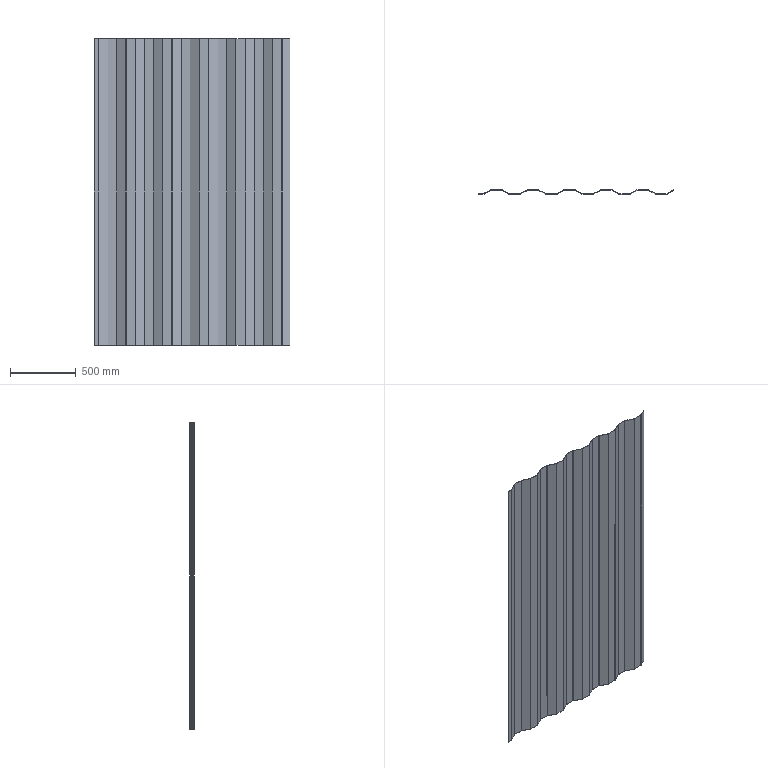Part | STEP file | 750038169 | 1 solid | 90 faces | box 1487 x 36 x 2327 mm | volume 7320463 mm3 | plane 48 | cylinder 42 | commonest cylinder face diameters 6 x21 10 x21